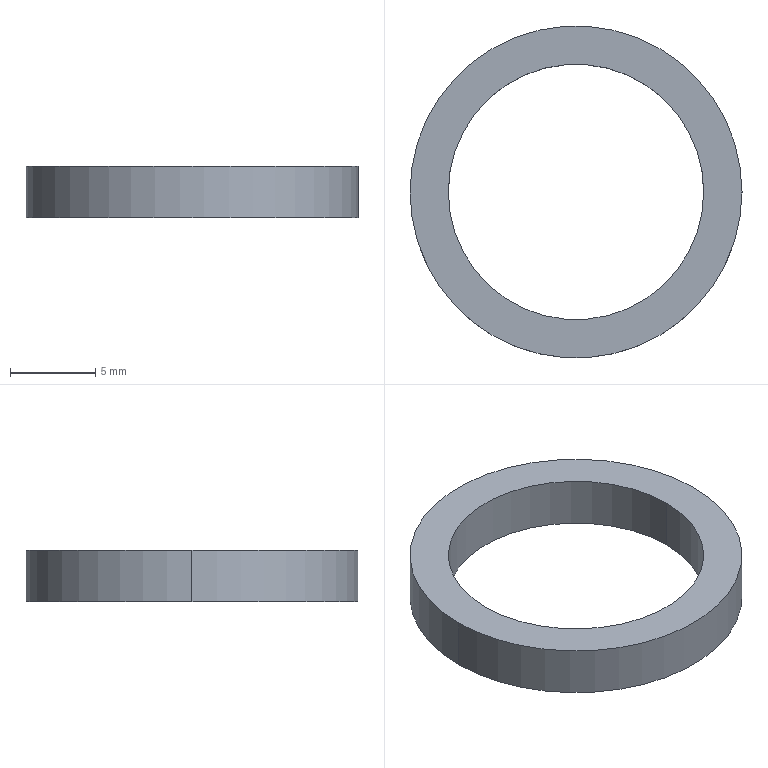Part | STEP file | PN_0051 retaining ring | 1 solid | 6 faces | box 19.5 x 19.5 x 3 mm | volume 365.799 mm3 | cylinder 4 | plane 2 | commonest cylinder face diameters 15 x2 19.5 x2
STEP:
#1=CARTESIAN_POINT('',(0.,0.,0.));
#2=DIRECTION('',(0.,0.,1.));
#3=DIRECTION('',(1.,0.,0.));
#4=AXIS2_PLACEMENT_3D('',#1,#2,#3);
#5=CARTESIAN_POINT('',(-7.5,0.,3.));
#6=VERTEX_POINT('',#5);
#7=CARTESIAN_POINT('',(-7.5,0.,0.));
#8=VERTEX_POINT('',#7);
#9=CARTESIAN_POINT('',(-7.5,0.,3.));
#10=DIRECTION('',(0.,0.,-1.));
#11=VECTOR('',#10,1.);
#12=LINE('',#9,#11);
#13=CARTESIAN_POINT('',(0.,0.,3.));
#14=DIRECTION('',(0.,0.,-1.));
#15=DIRECTION('',(-1.,0.,0.));
#16=AXIS2_PLACEMENT_3D('',#13,#14,#15);
#17=CYLINDRICAL_SURFACE('',#16,7.5);
#18=CARTESIAN_POINT('',(6.283,0.));
#19=DIRECTION('',(0.,1.));
#20=VECTOR('',#19,1.);
#21=LINE('',#18,#20);
#22=(GEOMETRIC_REPRESENTATION_CONTEXT(2)PARAMETRIC_REPRESENTATION_CONTEXT()REPRESENTATION_CONTEXT('',''));
#23=DEFINITIONAL_REPRESENTATION('',(#21),#22);
#24=PCURVE('',#17,#23);
#25=CARTESIAN_POINT('',(0.,0.,3.));
#26=DIRECTION('',(0.,0.,-1.));
#27=DIRECTION('',(-1.,0.,0.));
#28=AXIS2_PLACEMENT_3D('',#25,#26,#27);
#29=CYLINDRICAL_SURFACE('',#28,7.5);
#30=CARTESIAN_POINT('',(0.,0.));
#31=DIRECTION('',(0.,1.));
#32=VECTOR('',#31,1.);
#33=LINE('',#30,#32);
#34=(GEOMETRIC_REPRESENTATION_CONTEXT(2)PARAMETRIC_REPRESENTATION_CONTEXT()REPRESENTATION_CONTEXT('',''));
#35=DEFINITIONAL_REPRESENTATION('',(#33),#34);
#36=PCURVE('',#29,#35);
#37=SURFACE_CURVE('',#12,(#24,#36),.PCURVE_S1.);
#38=EDGE_CURVE('',#6,#8,#37,.T.);
#39=ORIENTED_EDGE('',*,*,#38,.T.);
#40=CARTESIAN_POINT('',(7.5,0.,0.));
#41=VERTEX_POINT('',#40);
#42=CARTESIAN_POINT('',(0.,0.,0.));
#43=DIRECTION('',(0.,0.,1.));
#44=DIRECTION('',(1.,0.,0.));
#45=AXIS2_PLACEMENT_3D('',#42,#43,#44);
#46=CIRCLE('',#45,7.5);
#47=CARTESIAN_POINT('',(9.425,3.));
#48=DIRECTION('',(-1.,0.));
#49=VECTOR('',#48,1.);
#50=LINE('',#47,#49);
#51=(GEOMETRIC_REPRESENTATION_CONTEXT(2)PARAMETRIC_REPRESENTATION_CONTEXT()REPRESENTATION_CONTEXT('',''));
#52=DEFINITIONAL_REPRESENTATION('',(#50),#51);
#53=PCURVE('',#17,#52);
#54=CARTESIAN_POINT('',(0.,0.,0.));
#55=DIRECTION('',(0.,0.,1.));
#56=DIRECTION('',(1.,0.,0.));
#57=AXIS2_PLACEMENT_3D('',#54,#55,#56);
#58=PLANE('',#57);
#59=CARTESIAN_POINT('',(0.,0.));
#60=DIRECTION('',(1.,0.));
#61=AXIS2_PLACEMENT_2D('',#59,#60);
#62=CIRCLE('',#61,7.5);
#63=(GEOMETRIC_REPRESENTATION_CONTEXT(2)PARAMETRIC_REPRESENTATION_CONTEXT()REPRESENTATION_CONTEXT('',''));
#64=DEFINITIONAL_REPRESENTATION('',(#62),#63);
#65=PCURVE('',#58,#64);
#66=SURFACE_CURVE('',#46,(#53,#65),.PCURVE_S1.);
#67=EDGE_CURVE('',#8,#41,#66,.T.);
#68=ORIENTED_EDGE('',*,*,#67,.T.);
#69=CARTESIAN_POINT('',(7.5,0.,3.));
#70=VERTEX_POINT('',#69);
#71=CARTESIAN_POINT('',(7.5,0.,3.));
#72=DIRECTION('',(0.,0.,-1.));
#73=VECTOR('',#72,1.);
#74=LINE('',#71,#73);
#75=CARTESIAN_POINT('',(3.142,0.));
#76=DIRECTION('',(0.,1.));
#77=VECTOR('',#76,1.);
#78=LINE('',#75,#77);
#79=(GEOMETRIC_REPRESENTATION_CONTEXT(2)PARAMETRIC_REPRESENTATION_CONTEXT()REPRESENTATION_CONTEXT('',''));
#80=DEFINITIONAL_REPRESENTATION('',(#78),#79);
#81=PCURVE('',#17,#80);
#82=CARTESIAN_POINT('',(3.142,0.));
#83=DIRECTION('',(0.,1.));
#84=VECTOR('',#83,1.);
#85=LINE('',#82,#84);
#86=(GEOMETRIC_REPRESENTATION_CONTEXT(2)PARAMETRIC_REPRESENTATION_CONTEXT()REPRESENTATION_CONTEXT('',''));
#87=DEFINITIONAL_REPRESENTATION('',(#85),#86);
#88=PCURVE('',#29,#87);
#89=SURFACE_CURVE('',#74,(#81,#88),.PCURVE_S1.);
#90=EDGE_CURVE('',#70,#41,#89,.T.);
#91=ORIENTED_EDGE('',*,*,#90,.F.);
#92=CARTESIAN_POINT('',(0.,0.,3.));
#93=DIRECTION('',(0.,0.,1.));
#94=DIRECTION('',(1.,0.,0.));
#95=AXIS2_PLACEMENT_3D('',#92,#93,#94);
#96=CIRCLE('',#95,7.5);
#97=CARTESIAN_POINT('',(9.425,0.));
#98=DIRECTION('',(-1.,0.));
#99=VECTOR('',#98,1.);
#100=LINE('',#97,#99);
#101=(GEOMETRIC_REPRESENTATION_CONTEXT(2)PARAMETRIC_REPRESENTATION_CONTEXT()REPRESENTATION_CONTEXT('',''));
#102=DEFINITIONAL_REPRESENTATION('',(#100),#101);
#103=PCURVE('',#17,#102);
#104=CARTESIAN_POINT('',(0.,0.,3.));
#105=DIRECTION('',(0.,0.,1.));
#106=DIRECTION('',(1.,0.,0.));
#107=AXIS2_PLACEMENT_3D('',#104,#105,#106);
#108=PLANE('',#107);
#109=CARTESIAN_POINT('',(0.,0.));
#110=DIRECTION('',(1.,0.));
#111=AXIS2_PLACEMENT_2D('',#109,#110);
#112=CIRCLE('',#111,7.5);
#113=(GEOMETRIC_REPRESENTATION_CONTEXT(2)PARAMETRIC_REPRESENTATION_CONTEXT()REPRESENTATION_CONTEXT('',''));
#114=DEFINITIONAL_REPRESENTATION('',(#112),#113);
#115=PCURVE('',#108,#114);
#116=SURFACE_CURVE('',#96,(#103,#115),.PCURVE_S1.);
#117=EDGE_CURVE('',#6,#70,#116,.T.);
#118=ORIENTED_EDGE('',*,*,#117,.F.);
#119=EDGE_LOOP('',(#39,#68,#91,#118));
#120=FACE_BOUND('',#119,.F.);
#121=ADVANCED_FACE('',(#120),#17,.F.);
#122=CARTESIAN_POINT('',(9.75,0.,3.));
#123=VERTEX_POINT('',#122);
#124=CARTESIAN_POINT('',(-9.75,0.,3.));
#125=VERTEX_POINT('',#124);
#126=CARTESIAN_POINT('',(0.,0.,3.));
#127=DIRECTION('',(0.,0.,1.));
#128=DIRECTION('',(1.,0.,0.));
#129=AXIS2_PLACEMENT_3D('',#126,#127,#128);
#130=CIRCLE('',#129,9.75);
#131=CARTESIAN_POINT('',(0.,0.,3.));
#132=DIRECTION('',(0.,0.,-1.));
#133=DIRECTION('',(-1.,0.,0.));
#134=AXIS2_PLACEMENT_3D('',#131,#132,#133);
#135=CYLINDRICAL_SURFACE('',#134,9.75);
#136=CARTESIAN_POINT('',(3.142,0.));
#137=DIRECTION('',(-1.,0.));
#138=VECTOR('',#137,1.);
#139=LINE('',#136,#138);
#140=(GEOMETRIC_REPRESENTATION_CONTEXT(2)PARAMETRIC_REPRESENTATION_CONTEXT()REPRESENTATION_CONTEXT('',''));
#141=DEFINITIONAL_REPRESENTATION('',(#139),#140);
#142=PCURVE('',#135,#141);
#143=CARTESIAN_POINT('',(0.,0.));
#144=DIRECTION('',(1.,0.));
#145=AXIS2_PLACEMENT_2D('',#143,#144);
#146=CIRCLE('',#145,9.75);
#147=(GEOMETRIC_REPRESENTATION_CONTEXT(2)PARAMETRIC_REPRESENTATION_CONTEXT()REPRESENTATION_CONTEXT('',''));
#148=DEFINITIONAL_REPRESENTATION('',(#146),#147);
#149=PCURVE('',#108,#148);
#150=SURFACE_CURVE('',#130,(#142,#149),.PCURVE_S1.);
#151=EDGE_CURVE('',#123,#125,#150,.T.);
#152=ORIENTED_EDGE('',*,*,#151,.F.);
#153=CARTESIAN_POINT('',(9.75,0.,0.));
#154=VERTEX_POINT('',#153);
#155=CARTESIAN_POINT('',(9.75,0.,3.));
#156=DIRECTION('',(0.,0.,-1.));
#157=VECTOR('',#156,1.);
#158=LINE('',#155,#157);
#159=CARTESIAN_POINT('',(3.142,0.));
#160=DIRECTION('',(0.,1.));
#161=VECTOR('',#160,1.);
#162=LINE('',#159,#161);
#163=(GEOMETRIC_REPRESENTATION_CONTEXT(2)PARAMETRIC_REPRESENTATION_CONTEXT()REPRESENTATION_CONTEXT('',''));
#164=DEFINITIONAL_REPRESENTATION('',(#162),#163);
#165=PCURVE('',#135,#164);
#166=CARTESIAN_POINT('',(0.,0.,3.));
#167=DIRECTION('',(0.,0.,-1.));
#168=DIRECTION('',(-1.,0.,0.));
#169=AXIS2_PLACEMENT_3D('',#166,#167,#168);
#170=CYLINDRICAL_SURFACE('',#169,9.75);
#171=CARTESIAN_POINT('',(3.142,0.));
#172=DIRECTION('',(0.,1.));
#173=VECTOR('',#172,1.);
#174=LINE('',#171,#173);
#175=(GEOMETRIC_REPRESENTATION_CONTEXT(2)PARAMETRIC_REPRESENTATION_CONTEXT()REPRESENTATION_CONTEXT('',''));
#176=DEFINITIONAL_REPRESENTATION('',(#174),#175);
#177=PCURVE('',#170,#176);
#178=SURFACE_CURVE('',#158,(#165,#177),.PCURVE_S1.);
#179=EDGE_CURVE('',#123,#154,#178,.T.);
#180=ORIENTED_EDGE('',*,*,#179,.T.);
#181=CARTESIAN_POINT('',(-9.75,0.,0.));
#182=VERTEX_POINT('',#181);
#183=CARTESIAN_POINT('',(0.,0.,0.));
#184=DIRECTION('',(0.,0.,1.));
#185=DIRECTION('',(1.,0.,0.));
#186=AXIS2_PLACEMENT_3D('',#183,#184,#185);
#187=CIRCLE('',#186,9.75);
#188=CARTESIAN_POINT('',(3.142,3.));
#189=DIRECTION('',(-1.,0.));
#190=VECTOR('',#189,1.);
#191=LINE('',#188,#190);
#192=(GEOMETRIC_REPRESENTATION_CONTEXT(2)PARAMETRIC_REPRESENTATION_CONTEXT()REPRESENTATION_CONTEXT('',''));
#193=DEFINITIONAL_REPRESENTATION('',(#191),#192);
#194=PCURVE('',#135,#193);
#195=CARTESIAN_POINT('',(0.,0.));
#196=DIRECTION('',(1.,0.));
#197=AXIS2_PLACEMENT_2D('',#195,#196);
#198=CIRCLE('',#197,9.75);
#199=(GEOMETRIC_REPRESENTATION_CONTEXT(2)PARAMETRIC_REPRESENTATION_CONTEXT()REPRESENTATION_CONTEXT('',''));
#200=DEFINITIONAL_REPRESENTATION('',(#198),#199);
#201=PCURVE('',#58,#200);
#202=SURFACE_CURVE('',#187,(#194,#201),.PCURVE_S1.);
#203=EDGE_CURVE('',#154,#182,#202,.T.);
#204=ORIENTED_EDGE('',*,*,#203,.T.);
#205=CARTESIAN_POINT('',(-9.75,0.,3.));
#206=DIRECTION('',(0.,0.,-1.));
#207=VECTOR('',#206,1.);
#208=LINE('',#205,#207);
#209=CARTESIAN_POINT('',(0.,0.));
#210=DIRECTION('',(0.,1.));
#211=VECTOR('',#210,1.);
#212=LINE('',#209,#211);
#213=(GEOMETRIC_REPRESENTATION_CONTEXT(2)PARAMETRIC_REPRESENTATION_CONTEXT()REPRESENTATION_CONTEXT('',''));
#214=DEFINITIONAL_REPRESENTATION('',(#212),#213);
#215=PCURVE('',#135,#214);
#216=CARTESIAN_POINT('',(6.283,0.));
#217=DIRECTION('',(0.,1.));
#218=VECTOR('',#217,1.);
#219=LINE('',#216,#218);
#220=(GEOMETRIC_REPRESENTATION_CONTEXT(2)PARAMETRIC_REPRESENTATION_CONTEXT()REPRESENTATION_CONTEXT('',''));
#221=DEFINITIONAL_REPRESENTATION('',(#219),#220);
#222=PCURVE('',#170,#221);
#223=SURFACE_CURVE('',#208,(#215,#222),.PCURVE_S1.);
#224=EDGE_CURVE('',#125,#182,#223,.T.);
#225=ORIENTED_EDGE('',*,*,#224,.F.);
#226=EDGE_LOOP('',(#152,#180,#204,#225));
#227=FACE_BOUND('',#226,.T.);
#228=ADVANCED_FACE('',(#227),#135,.T.);
#229=CARTESIAN_POINT('',(0.,0.,3.));
#230=DIRECTION('',(0.,0.,1.));
#231=DIRECTION('',(1.,0.,0.));
#232=AXIS2_PLACEMENT_3D('',#229,#230,#231);
#233=CIRCLE('',#232,9.75);
#234=CARTESIAN_POINT('',(0.,0.));
#235=DIRECTION('',(1.,0.));
#236=AXIS2_PLACEMENT_2D('',#234,#235);
#237=CIRCLE('',#236,9.75);
#238=(GEOMETRIC_REPRESENTATION_CONTEXT(2)PARAMETRIC_REPRESENTATION_CONTEXT()REPRESENTATION_CONTEXT('',''));
#239=DEFINITIONAL_REPRESENTATION('',(#237),#238);
#240=PCURVE('',#108,#239);
#241=CARTESIAN_POINT('',(9.425,0.));
#242=DIRECTION('',(-1.,0.));
#243=VECTOR('',#242,1.);
#244=LINE('',#241,#243);
#245=(GEOMETRIC_REPRESENTATION_CONTEXT(2)PARAMETRIC_REPRESENTATION_CONTEXT()REPRESENTATION_CONTEXT('',''));
#246=DEFINITIONAL_REPRESENTATION('',(#244),#245);
#247=PCURVE('',#170,#246);
#248=SURFACE_CURVE('',#233,(#240,#247),.PCURVE_S1.);
#249=EDGE_CURVE('',#125,#123,#248,.T.);
#250=ORIENTED_EDGE('',*,*,#249,.T.);
#251=ORIENTED_EDGE('',*,*,#151,.T.);
#252=EDGE_LOOP('',(#250,#251));
#253=FACE_BOUND('',#252,.T.);
#254=ORIENTED_EDGE('',*,*,#117,.F.);
#255=CARTESIAN_POINT('',(0.,0.,3.));
#256=DIRECTION('',(0.,0.,1.));
#257=DIRECTION('',(1.,0.,0.));
#258=AXIS2_PLACEMENT_3D('',#255,#256,#257);
#259=CIRCLE('',#258,7.5);
#260=CARTESIAN_POINT('',(0.,0.));
#261=DIRECTION('',(1.,0.));
#262=AXIS2_PLACEMENT_2D('',#260,#261);
#263=CIRCLE('',#262,7.5);
#264=(GEOMETRIC_REPRESENTATION_CONTEXT(2)PARAMETRIC_REPRESENTATION_CONTEXT()REPRESENTATION_CONTEXT('',''));
#265=DEFINITIONAL_REPRESENTATION('',(#263),#264);
#266=PCURVE('',#108,#265);
#267=CARTESIAN_POINT('',(3.142,0.));
#268=DIRECTION('',(-1.,0.));
#269=VECTOR('',#268,1.);
#270=LINE('',#267,#269);
#271=(GEOMETRIC_REPRESENTATION_CONTEXT(2)PARAMETRIC_REPRESENTATION_CONTEXT()REPRESENTATION_CONTEXT('',''));
#272=DEFINITIONAL_REPRESENTATION('',(#270),#271);
#273=PCURVE('',#29,#272);
#274=SURFACE_CURVE('',#259,(#266,#273),.PCURVE_S1.);
#275=EDGE_CURVE('',#70,#6,#274,.T.);
#276=ORIENTED_EDGE('',*,*,#275,.F.);
#277=EDGE_LOOP('',(#254,#276));
#278=FACE_BOUND('',#277,.T.);
#279=ADVANCED_FACE('',(#253,#278),#108,.T.);
#280=CARTESIAN_POINT('',(0.,0.,0.));
#281=DIRECTION('',(0.,0.,1.));
#282=DIRECTION('',(1.,0.,0.));
#283=AXIS2_PLACEMENT_3D('',#280,#281,#282);
#284=CIRCLE('',#283,9.75);
#285=CARTESIAN_POINT('',(0.,0.));
#286=DIRECTION('',(1.,0.));
#287=AXIS2_PLACEMENT_2D('',#285,#286);
#288=CIRCLE('',#287,9.75);
#289=(GEOMETRIC_REPRESENTATION_CONTEXT(2)PARAMETRIC_REPRESENTATION_CONTEXT()REPRESENTATION_CONTEXT('',''));
#290=DEFINITIONAL_REPRESENTATION('',(#288),#289);
#291=PCURVE('',#58,#290);
#292=CARTESIAN_POINT('',(9.425,3.));
#293=DIRECTION('',(-1.,0.));
#294=VECTOR('',#293,1.);
#295=LINE('',#292,#294);
#296=(GEOMETRIC_REPRESENTATION_CONTEXT(2)PARAMETRIC_REPRESENTATION_CONTEXT()REPRESENTATION_CONTEXT('',''));
#297=DEFINITIONAL_REPRESENTATION('',(#295),#296);
#298=PCURVE('',#170,#297);
#299=SURFACE_CURVE('',#284,(#291,#298),.PCURVE_S1.);
#300=EDGE_CURVE('',#182,#154,#299,.T.);
#301=ORIENTED_EDGE('',*,*,#300,.F.);
#302=ORIENTED_EDGE('',*,*,#203,.F.);
#303=EDGE_LOOP('',(#301,#302));
#304=FACE_BOUND('',#303,.T.);
#305=ORIENTED_EDGE('',*,*,#67,.T.);
#306=CARTESIAN_POINT('',(0.,0.,0.));
#307=DIRECTION('',(0.,0.,1.));
#308=DIRECTION('',(1.,0.,0.));
#309=AXIS2_PLACEMENT_3D('',#306,#307,#308);
#310=CIRCLE('',#309,7.5);
#311=CARTESIAN_POINT('',(0.,0.));
#312=DIRECTION('',(1.,0.));
#313=AXIS2_PLACEMENT_2D('',#311,#312);
#314=CIRCLE('',#313,7.5);
#315=(GEOMETRIC_REPRESENTATION_CONTEXT(2)PARAMETRIC_REPRESENTATION_CONTEXT()REPRESENTATION_CONTEXT('',''));
#316=DEFINITIONAL_REPRESENTATION('',(#314),#315);
#317=PCURVE('',#58,#316);
#318=CARTESIAN_POINT('',(3.142,3.));
#319=DIRECTION('',(-1.,0.));
#320=VECTOR('',#319,1.);
#321=LINE('',#318,#320);
#322=(GEOMETRIC_REPRESENTATION_CONTEXT(2)PARAMETRIC_REPRESENTATION_CONTEXT()REPRESENTATION_CONTEXT('',''));
#323=DEFINITIONAL_REPRESENTATION('',(#321),#322);
#324=PCURVE('',#29,#323);
#325=SURFACE_CURVE('',#310,(#317,#324),.PCURVE_S1.);
#326=EDGE_CURVE('',#41,#8,#325,.T.);
#327=ORIENTED_EDGE('',*,*,#326,.T.);
#328=EDGE_LOOP('',(#305,#327));
#329=FACE_BOUND('',#328,.T.);
#330=ADVANCED_FACE('',(#304,#329),#58,.F.);
#331=ORIENTED_EDGE('',*,*,#179,.F.);
#332=ORIENTED_EDGE('',*,*,#249,.F.);
#333=ORIENTED_EDGE('',*,*,#224,.T.);
#334=ORIENTED_EDGE('',*,*,#300,.T.);
#335=EDGE_LOOP('',(#331,#332,#333,#334));
#336=FACE_BOUND('',#335,.T.);
#337=ADVANCED_FACE('',(#336),#170,.T.);
#338=ORIENTED_EDGE('',*,*,#326,.T.);
#339=ORIENTED_EDGE('',*,*,#38,.F.);
#340=ORIENTED_EDGE('',*,*,#275,.F.);
#341=ORIENTED_EDGE('',*,*,#90,.T.);
#342=EDGE_LOOP('',(#338,#339,#340,#341));
#343=FACE_BOUND('',#342,.F.);
#344=ADVANCED_FACE('',(#343),#29,.F.);
#345=CLOSED_SHELL('',(#121,#228,#279,#330,#337,#344));
#346=MANIFOLD_SOLID_BREP('',#345);
#347=(LENGTH_UNIT()NAMED_UNIT(*)SI_UNIT(.MILLI.,.METRE.));
#348=UNCERTAINTY_MEASURE_WITH_UNIT(LENGTH_MEASURE(0.0000001),#347,'','');
#349=(NAMED_UNIT(*)PLANE_ANGLE_UNIT()SI_UNIT($,.RADIAN.));
#350=(NAMED_UNIT(*)SI_UNIT($,.STERADIAN.)SOLID_ANGLE_UNIT());
#351=(GEOMETRIC_REPRESENTATION_CONTEXT(3)GLOBAL_UNCERTAINTY_ASSIGNED_CONTEXT((#348))GLOBAL_UNIT_ASSIGNED_CONTEXT((#347,#349,#350))REPRESENTATION_CONTEXT('',''));
#352=ADVANCED_BREP_SHAPE_REPRESENTATION('',(#4,#346),#351);